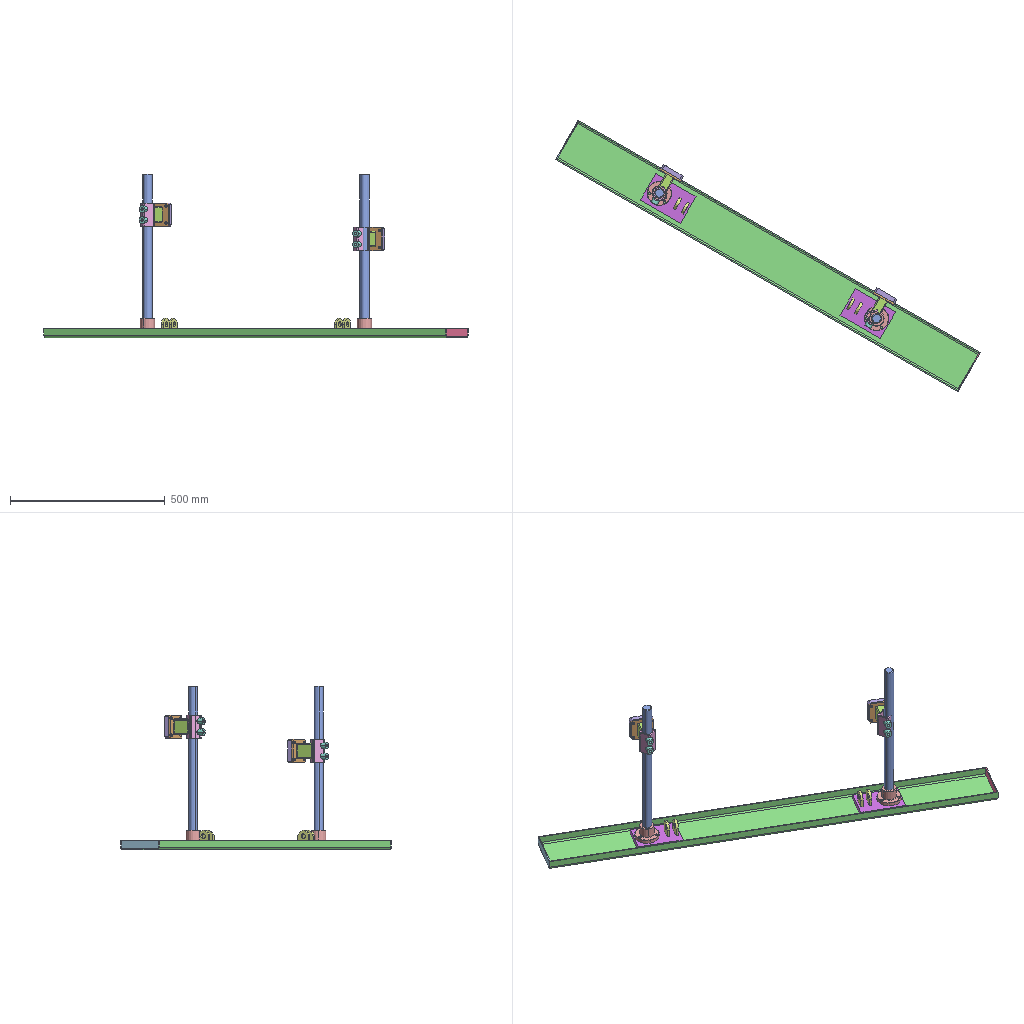Assembly | SolidWorks | 13 different items | 28 placed | box 1372 x 876 x 528 mm
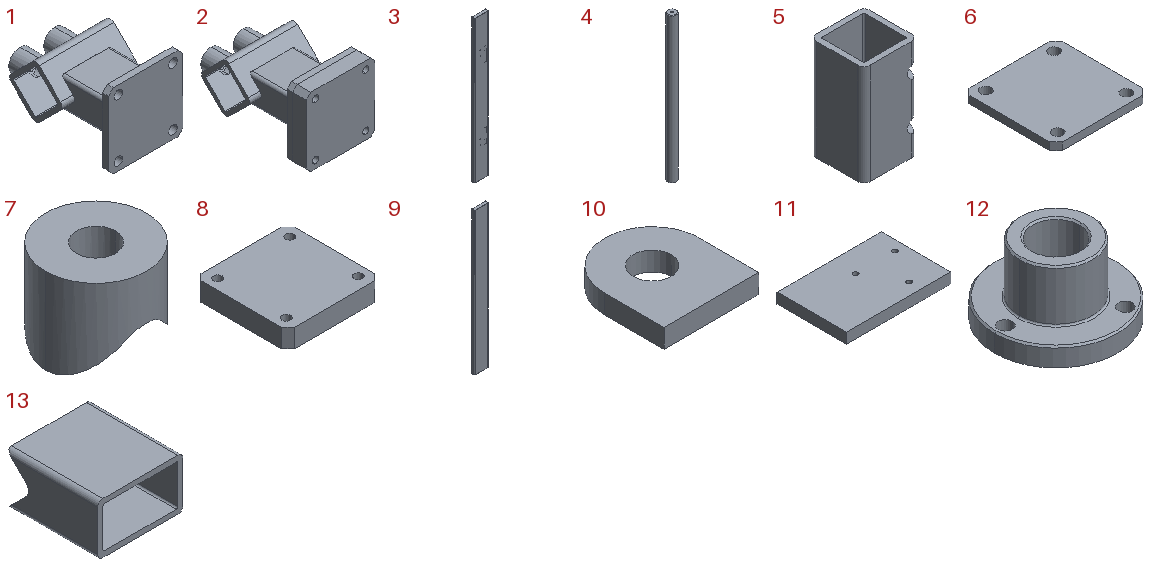Parts list (item | name | quantity | parent item | size | volume | features):
1 | (subassembly) | x2 | in 2 | 75 x 109 x 75 mm | 103029 mm3 | -
2 | (subassembly) | x2 | - | 75 x 124 x 75 mm | 184475 mm3 | -
3 | (subassembly) | x1 | - | 145 x 63 x 1500 mm | 1385163 mm3 | features CompositeCurve 1
4 | - | x2 | - | 30 x 30 x 500 mm | 351630 mm3 | features Chamfer 1, Extrusion 1, HoleWzd 1
5 | - | x2 | in 1 | 40 x 40 x 75 mm | 40690 mm3 | features Extrusion 1, ICE 1
6 | - | x2 | in 1 | 75 x 75 x 6 mm | 32088 mm3 | features Extrusion 1
7 | - | x4 | in 1 | 22 x 22 x 18.716 mm | 4241 mm3 | features Extrusion 1, HoleWzd 1, ICE 1
8 | - | x2 | in 2 | 75 x 75 x 15 mm | 81446 mm3 | features Extrusion 1, HoleWzd 1
9 | - | x1 | in 3 | 145 x 30 x 1500 mm | 892760 mm3 | features ICE 2, Extrusion 1
10 | - | x4 | in 3 | 40 x 45 x 8 mm | 11418 mm3 | features Extrusion 1
11 | - | x2 | in 3 | 150 x 100 x 15 mm | 223366 mm3 | features Extrusion 1, HoleWzd 1
12 | - | x2 | - | 79 x 79 x 45 mm | 86695 mm3 | features ICE 5, Chamfer 1, Extrusion 1, Fillet 1
13 | - | x2 | in 1 | 50 x 53.7 x 30 mm | 21768 mm3 | features Fillet 2, Extrusion 1, ICE 1, Shell 1
Mates (type | each side: item.copy, entity, surface, feature):
In the top assembly
Coincident | 12.1 face plane Cut-Extrude1 | 4.1 face plane Boss-Extrude1
Concentric | 12.1 face cylinder Boss-Extrude1 | 4.1 face cylinder Boss-Extrude1
Coincident | 4.2 face plane Boss-Extrude1 | 12.2 face plane Cut-Extrude1
Concentric | 4.2 face cylinder Boss-Extrude1 | 12.2 face cylinder Boss-Extrude2
Coincident | 12.1 face plane Boss-Extrude1 | 12.2 face plane Boss-Extrude1
Parallel | 12.2 face plane Boss-Extrude1 | 5.1 face plane Boss-Extrude1
Coincident | 6.1 face plane Boss-Extrude1 | 6.2 face plane Boss-Extrude1
Coincident | 12.2 face plane Boss-Extrude1 | 11.1 face plane Boss-Extrude1
Concentric | 12.2 face cylinder Cut-Extrude4 | 11.1 face cylinder M8 Tapped Hole1 | 2 times
Parallel | 6.2 face plane Boss-Extrude1 | 9.1 face plane Boss-Extrude1
Concentric | 12.1 face cylinder Cut-Extrude4 | 11.2 face cylinder M8 Tapped Hole1 | 2 times
In subassembly 2
Coincident | 6.3 face plane Boss-Extrude1 | 8.1 face plane Boss-Extrude1
Concentric | 6.3 face cylinder Boss-Extrude1 | 8.1 face cylinder M8 Tapped Hole1 | 2 times
In subassembly 1
Concentric | 5.2 face cylinder Cut-Extrude1 | 7.1 face cylinder M10 Tapped Hole1
Coincident | 5.2 face plane Boss-Extrude1 | 7.1 face plane Cut-Extrude1
Concentric | 13.1 face cylinder Cut-Extrude1 | 5.2 face cylinder Boss-Extrude1
Coincident | 13.1 face plane Cut-Extrude1 | 5.2 face plane Boss-Extrude1
Width | 5.2 face plane Boss-Extrude1 | 5.2 face plane Boss-Extrude1 | 13.1 face plane Boss-Extrude1 | 13.1 face plane Boss-Extrude1
Concentric | 5.2 face cylinder Cut-Extrude1 | 7.2 face cylinder M10 Tapped Hole1
Coincident | 5.2 face plane Boss-Extrude1 | 7.2 face plane Cut-Extrude1
Coincident | 13.1 face plane Boss-Extrude1 | 6.4 face plane Boss-Extrude1
Width | 13.1 face plane Boss-Extrude1 | 13.1 face plane Boss-Extrude1 | 6.4 face plane Boss-Extrude1 | 6.4 face plane Boss-Extrude1 | 2 times
In subassembly 3
Coincident | 9.2 face plane Boss-Extrude1 | 11.3 face plane Boss-Extrude1
Parallel | 9.2 face plane Boss-Extrude1 | 11.3 face plane Boss-Extrude1
Width | 9.2 face plane Boss-Extrude1 | 9.2 face plane Boss-Extrude1 | 11.3 face plane Boss-Extrude1 | 11.3 face plane Boss-Extrude1
Coincident | 11.3 face plane Boss-Extrude1 | 11.4 face plane Boss-Extrude1 | 2 times
Coincident | 10.1 face plane Boss-Extrude1 | 11.3 face plane Boss-Extrude1
DistanceDim | 10.1 face plane Boss-Extrude1 | 11.3 face plane Boss-Extrude1
Width | 10.1 face plane Boss-Extrude1 | 10.1 face plane Boss-Extrude1 | 11.3 face plane Boss-Extrude1 | 11.3 face plane Boss-Extrude1
Coincident | 10.2 face plane Boss-Extrude1 | 10.3 face plane Boss-Extrude1 | 2 times
Coincident | 10.4 face plane Boss-Extrude1 | 10.3 face plane Boss-Extrude1
Coincident | 10.1 face plane Boss-Extrude1 | 10.3 face plane Boss-Extrude1
Coincident | 10.4 face plane Boss-Extrude1 | 10.2 face plane Boss-Extrude1
Coincident | 11.3 face plane Boss-Extrude1 | 10.3 face plane Boss-Extrude1
DistanceDim | 10.3 face plane Boss-Extrude1 | 10.1 face plane Boss-Extrude1
DistanceDim | 10.2 face plane Boss-Extrude1 | 11.4 face plane Boss-Extrude1
DistanceDim | 10.4 face plane Boss-Extrude1 | 10.2 face plane Boss-Extrude1
DistanceDim | 11.4 face plane Boss-Extrude1 | 11.3 face plane Boss-Extrude1
DistanceDim | 11.4 face plane Boss-Extrude1 | 9.2 face plane Boss-Extrude2